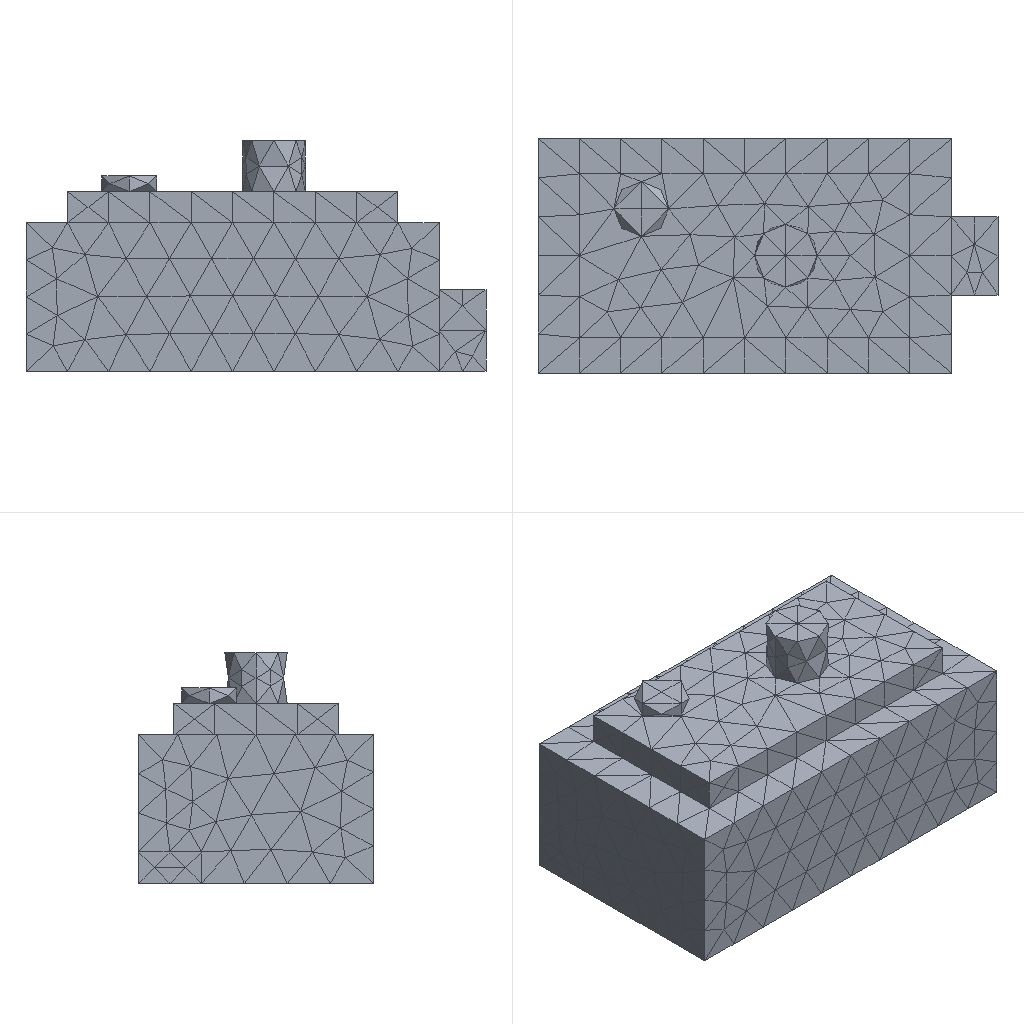Simulation study | ansys mapdl
Set-up summary:
category,name,step,type,value,unit,region
solver,ansys_mapdl
units,mm-N-s-tonne (MPa),,inferred,E=210000 density=
analysis,model,,static
mesh,nodes,,,3939
mesh,elements,,,2314
element_type,SOLID187,,,2314
material,mat 1,,E,210000
material,mat 1,,nu,0.3
load,,model,body load temp,,,all
load,,model,force,"1000 [dir=(0, 0, -1) n=186]",,node list
bc,,model,fixed,"[dofs=UX,UY,UZ n=4269]",,node list
Ansys APDL input file, long lists of numbers shortened:
/COM,ANSYS RELEASE 2026 R1           BUILD 26.1      UP20260202       09:09:04
/PREP7
/NOPR
/TITLE,2
ANTYPE, 0
*IF,_CDRDOFF,EQ,1,THEN     !if solid model was read in
_CDRDOFF=             !reset flag, numoffs already performed
*ELSE              !offset database for the following FE model
NUMOFF,NODE,     3939
NUMOFF,ELEM,     2314
NUMOFF,MAT ,        1
NUMOFF,TYPE,        1
*ENDIF
*SET,_RETURN ,  0.
*SET,_STATUS ,  0.
*SET,_UIQR   ,  186.
*SET,__FLOATPARAMETER__,  3939.
DOF,DELETE
ETBLOCK,        1,        1
(2i9,19a9)
        1      187        0        0        0        0        0        0        0        0        0        0        0        0        0        0        0        0        0        0        0
       -1
NBLOCK,6,SOLID,      3939,      3939
(3i9,6e21.13e3)
        1        0        0-3.6875000000000E+001 3.0000000000000E+001 8.0000000000000E+000
! (3938 more lines like these left out)
N,UNBL,LOC,       -1,
EBLOCK,19,SOLID,      2314,      2314
(19i10)
         1         1         1         1         0         0         0         0        10         0         1      1611      1612       622       440      1819      1820      1821      1822
! (4627 more lines like these left out)
        -1
MPTEMP,UNBL, 1, 1,  0.    ,
MPDATA,UNBL, 1,EX  ,       1, 1,  210000.000    ,
MPTEMP,UNBL, 1, 1,  0.    ,
MPDATA,UNBL, 1,NUXY,       1, 1, 0.3    ,
MPTEMP,UNBL, 1, 1,  0.    ,
MPDATA,UNBL, 1,PRXY,       1, 1, 0.3    ,
EXTOPT,ATTR,      0,      0,      0
EXTOPT,ESIZE,  0,  0.
EXTOPT,ACLEAR,      0
TREF,  0.
IRLF,  0
BFUNIF,TEMP,_TINY
ACEL,  0.    ,  0.    ,  0.
OMEGA,  0.    ,  0.    ,  0.
DOMEGA,  0.    ,  0.    ,  0.
CGLOC,  0.    ,  0.    ,  0.
CGOMEGA,  0.    ,  0.    ,  0.
DCGOMG,  0.    ,  0.    ,  0.
KUSE,     0
TIME,  0.
ALPHAD,  0.
BETAD,  0.
DMPRAT,  0.
DMPSTR,  0.
CRPLIM, 0.1    ,   0
CRPLIM,  0.    ,   1
NCNV,     0, 1.000000000E+12,     0,  0.    ,  0.
NEQIT,     0
ERESX,DEFA
DBLOCK,      4269
(i9,a6,2(pg16.9))
        1  UX    0.00000000      0.00000000
! (4268 more lines like these left out)
       -1
FBLOCK,       186
(i9,a6,2(pg16.9))
      777  FZ   -5.37634409      0.00000000
! (185 more lines like these left out)
       -1
/GO
FINISH
Results summary:
result,analysis_type_db,,,static,unstated
result,n_sets,,,1,unstated
result,load_steps[0].set,load_step=1,,1,unstated
result,load_steps[0].substep,load_step=1,,1,unstated
result,load_steps[0].time,load_step=1,,1,unstated
result,load_steps[0].freq,load_step=1,,1,unstated
result,load_steps[0].max_usum,load_step=1,,0.0004094,unstated
result,load_steps[0].max_seqv,load_step=1,,4.878,unstated
result,load_steps[0].reaction_sum.FX,load_step=1,,5.32552e-12,unstated
result,load_steps[0].reaction_sum.FY,load_step=1,,5.11635e-12,unstated
result,load_steps[0].reaction_sum.FZ,load_step=1,,1000,unstated
result,load_steps[0].reaction_sum.MX,load_step=1,,0,unstated
result,load_steps[0].reaction_sum.MY,load_step=1,,0,unstated
result,load_steps[0].reaction_sum.MZ,load_step=1,,0,unstated
result,convergence,,,results present for all listed sets,unstated